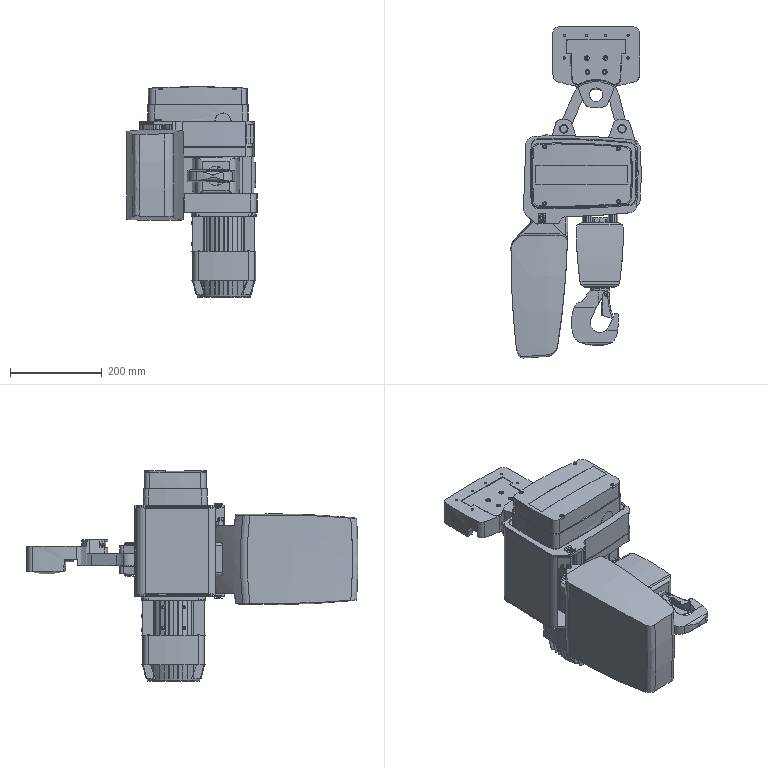Part | SolidWorks | features BaseBody 17, Scale 1 | 17 solids | 2032 faces | box 284.321 x 725.83 x 459.6 mm | volume 19917638 mm3 | plane 1063 | cylinder 683 | torus 148 | cone 134 | sphere 4 | commonest cylinder face diameters 7.5 x64 4.5 x37 117.75 x32 9 x27 12 x27 6.75 x24